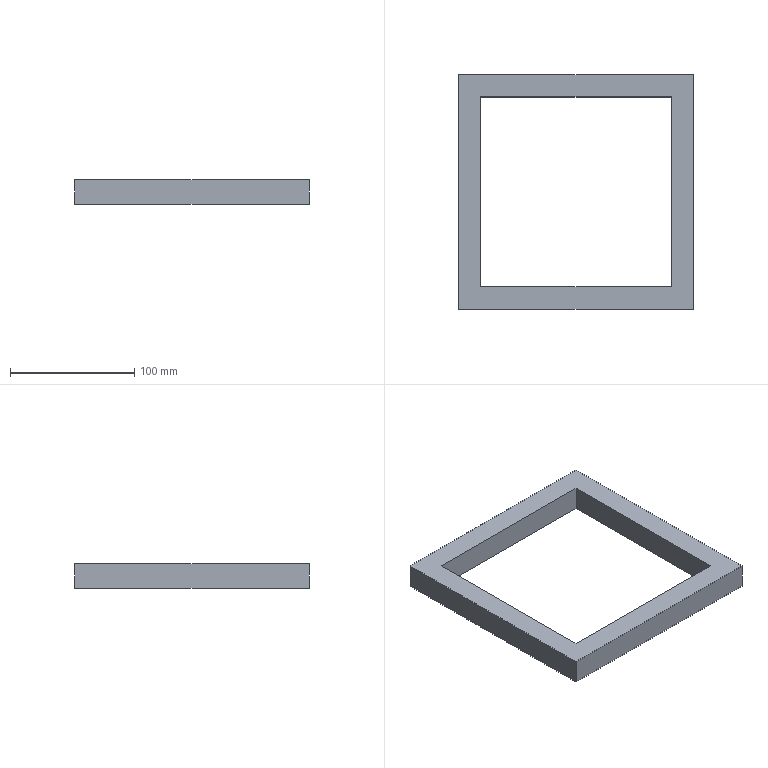Part | SolidWorks | features BaseBody 1 | 1 solid | 10 faces | box 189 x 189 x 20 mm | volume 246240 mm3 | plane 10
STEP:
#1=CARTESIAN_POINT('',(-76.5,-76.5,0.));
#2=VERTEX_POINT('',#1);
#3=CARTESIAN_POINT('',(76.5,-76.5,0.));
#4=VERTEX_POINT('',#3);
#5=CARTESIAN_POINT('',(76.5,-76.5,0.));
#6=DIRECTION('',(1.,0.,0.));
#7=VECTOR('',#6,1000.);
#8=LINE('',#5,#7);
#9=EDGE_CURVE('',#2,#4,#8,.T.);
#10=ORIENTED_EDGE('',*,*,#9,.F.);
#11=CARTESIAN_POINT('',(-76.5,-76.5,20.));
#12=VERTEX_POINT('',#11);
#13=CARTESIAN_POINT('',(-76.5,-76.5,20.));
#14=DIRECTION('',(0.,0.,-1.));
#15=VECTOR('',#14,1000.);
#16=LINE('',#13,#15);
#17=EDGE_CURVE('',#12,#2,#16,.T.);
#18=ORIENTED_EDGE('',*,*,#17,.F.);
#19=CARTESIAN_POINT('',(76.5,-76.5,20.));
#20=VERTEX_POINT('',#19);
#21=CARTESIAN_POINT('',(76.5,-76.5,20.));
#22=DIRECTION('',(1.,0.,0.));
#23=VECTOR('',#22,1000.);
#24=LINE('',#21,#23);
#25=EDGE_CURVE('',#12,#20,#24,.T.);
#26=ORIENTED_EDGE('',*,*,#25,.T.);
#27=CARTESIAN_POINT('',(76.5,-76.5,20.));
#28=DIRECTION('',(0.,0.,-1.));
#29=VECTOR('',#28,1000.);
#30=LINE('',#27,#29);
#31=EDGE_CURVE('',#20,#4,#30,.T.);
#32=ORIENTED_EDGE('',*,*,#31,.T.);
#33=EDGE_LOOP('',(#10,#18,#26,#32));
#34=FACE_OUTER_BOUND('',#33,.T.);
#35=CARTESIAN_POINT('',(76.5,-76.5,20.));
#36=DIRECTION('',(0.,1.,0.));
#37=DIRECTION('',(1.,0.,0.));
#38=AXIS2_PLACEMENT_3D('',#35,#36,#37);
#39=PLANE('',#38);
#40=ADVANCED_FACE('',(#34),#39,.T.);
#41=CARTESIAN_POINT('',(-76.5,76.5,0.));
#42=VERTEX_POINT('',#41);
#43=CARTESIAN_POINT('',(-76.5,76.5,0.));
#44=DIRECTION('',(0.,-1.,0.));
#45=VECTOR('',#44,1000.);
#46=LINE('',#43,#45);
#47=EDGE_CURVE('',#42,#2,#46,.T.);
#48=ORIENTED_EDGE('',*,*,#47,.F.);
#49=CARTESIAN_POINT('',(-76.5,76.5,20.));
#50=VERTEX_POINT('',#49);
#51=CARTESIAN_POINT('',(-76.5,76.5,20.));
#52=DIRECTION('',(0.,0.,-1.));
#53=VECTOR('',#52,1000.);
#54=LINE('',#51,#53);
#55=EDGE_CURVE('',#50,#42,#54,.T.);
#56=ORIENTED_EDGE('',*,*,#55,.F.);
#57=CARTESIAN_POINT('',(-76.5,76.5,20.));
#58=DIRECTION('',(0.,-1.,0.));
#59=VECTOR('',#58,1000.);
#60=LINE('',#57,#59);
#61=EDGE_CURVE('',#50,#12,#60,.T.);
#62=ORIENTED_EDGE('',*,*,#61,.T.);
#63=ORIENTED_EDGE('',*,*,#17,.T.);
#64=EDGE_LOOP('',(#48,#56,#62,#63));
#65=FACE_OUTER_BOUND('',#64,.T.);
#66=CARTESIAN_POINT('',(-76.5,76.5,20.));
#67=DIRECTION('',(1.,0.,0.));
#68=DIRECTION('',(0.,1.,0.));
#69=AXIS2_PLACEMENT_3D('',#66,#67,#68);
#70=PLANE('',#69);
#71=ADVANCED_FACE('',(#65),#70,.T.);
#72=CARTESIAN_POINT('',(76.5,76.5,0.));
#73=VERTEX_POINT('',#72);
#74=CARTESIAN_POINT('',(76.5,76.5,0.));
#75=DIRECTION('',(-1.,0.,0.));
#76=VECTOR('',#75,1000.);
#77=LINE('',#74,#76);
#78=EDGE_CURVE('',#73,#42,#77,.T.);
#79=ORIENTED_EDGE('',*,*,#78,.F.);
#80=CARTESIAN_POINT('',(76.5,76.5,20.));
#81=VERTEX_POINT('',#80);
#82=CARTESIAN_POINT('',(76.5,76.5,20.));
#83=DIRECTION('',(0.,0.,-1.));
#84=VECTOR('',#83,1000.);
#85=LINE('',#82,#84);
#86=EDGE_CURVE('',#81,#73,#85,.T.);
#87=ORIENTED_EDGE('',*,*,#86,.F.);
#88=CARTESIAN_POINT('',(76.5,76.5,20.));
#89=DIRECTION('',(-1.,0.,0.));
#90=VECTOR('',#89,1000.);
#91=LINE('',#88,#90);
#92=EDGE_CURVE('',#81,#50,#91,.T.);
#93=ORIENTED_EDGE('',*,*,#92,.T.);
#94=ORIENTED_EDGE('',*,*,#55,.T.);
#95=EDGE_LOOP('',(#79,#87,#93,#94));
#96=FACE_OUTER_BOUND('',#95,.T.);
#97=CARTESIAN_POINT('',(76.5,76.5,20.));
#98=DIRECTION('',(0.,-1.,0.));
#99=DIRECTION('',(0.,0.,-1.));
#100=AXIS2_PLACEMENT_3D('',#97,#98,#99);
#101=PLANE('',#100);
#102=ADVANCED_FACE('',(#96),#101,.T.);
#103=CARTESIAN_POINT('',(76.5,76.5,0.));
#104=DIRECTION('',(0.,1.,0.));
#105=VECTOR('',#104,1000.);
#106=LINE('',#103,#105);
#107=EDGE_CURVE('',#4,#73,#106,.T.);
#108=ORIENTED_EDGE('',*,*,#107,.F.);
#109=ORIENTED_EDGE('',*,*,#31,.F.);
#110=CARTESIAN_POINT('',(76.5,76.5,20.));
#111=DIRECTION('',(0.,1.,0.));
#112=VECTOR('',#111,1000.);
#113=LINE('',#110,#112);
#114=EDGE_CURVE('',#20,#81,#113,.T.);
#115=ORIENTED_EDGE('',*,*,#114,.T.);
#116=ORIENTED_EDGE('',*,*,#86,.T.);
#117=EDGE_LOOP('',(#108,#109,#115,#116));
#118=FACE_OUTER_BOUND('',#117,.T.);
#119=CARTESIAN_POINT('',(76.5,76.5,20.));
#120=DIRECTION('',(-1.,0.,0.));
#121=DIRECTION('',(0.,1.,0.));
#122=AXIS2_PLACEMENT_3D('',#119,#120,#121);
#123=PLANE('',#122);
#124=ADVANCED_FACE('',(#118),#123,.T.);
#125=CARTESIAN_POINT('',(94.5,94.5,0.));
#126=VERTEX_POINT('',#125);
#127=CARTESIAN_POINT('',(-94.5,94.5,0.));
#128=VERTEX_POINT('',#127);
#129=CARTESIAN_POINT('',(94.5,94.5,0.));
#130=DIRECTION('',(-1.,0.,0.));
#131=VECTOR('',#130,1000.);
#132=LINE('',#129,#131);
#133=EDGE_CURVE('',#126,#128,#132,.T.);
#134=ORIENTED_EDGE('',*,*,#133,.T.);
#135=CARTESIAN_POINT('',(-94.5,94.5,20.));
#136=VERTEX_POINT('',#135);
#137=CARTESIAN_POINT('',(-94.5,94.5,20.));
#138=DIRECTION('',(0.,0.,-1.));
#139=VECTOR('',#138,1000.);
#140=LINE('',#137,#139);
#141=EDGE_CURVE('',#136,#128,#140,.T.);
#142=ORIENTED_EDGE('',*,*,#141,.F.);
#143=CARTESIAN_POINT('',(94.5,94.5,20.));
#144=VERTEX_POINT('',#143);
#145=CARTESIAN_POINT('',(94.5,94.5,20.));
#146=DIRECTION('',(-1.,0.,0.));
#147=VECTOR('',#146,1000.);
#148=LINE('',#145,#147);
#149=EDGE_CURVE('',#144,#136,#148,.T.);
#150=ORIENTED_EDGE('',*,*,#149,.F.);
#151=CARTESIAN_POINT('',(94.5,94.5,20.));
#152=DIRECTION('',(0.,0.,-1.));
#153=VECTOR('',#152,1000.);
#154=LINE('',#151,#153);
#155=EDGE_CURVE('',#144,#126,#154,.T.);
#156=ORIENTED_EDGE('',*,*,#155,.T.);
#157=EDGE_LOOP('',(#134,#142,#150,#156));
#158=FACE_OUTER_BOUND('',#157,.T.);
#159=CARTESIAN_POINT('',(94.5,94.5,20.));
#160=DIRECTION('',(0.,-1.,0.));
#161=DIRECTION('',(0.,0.,-1.));
#162=AXIS2_PLACEMENT_3D('',#159,#160,#161);
#163=PLANE('',#162);
#164=ADVANCED_FACE('',(#158),#163,.F.);
#165=CARTESIAN_POINT('',(94.5,-94.5,0.));
#166=VERTEX_POINT('',#165);
#167=CARTESIAN_POINT('',(94.5,94.5,0.));
#168=DIRECTION('',(0.,1.,0.));
#169=VECTOR('',#168,1000.);
#170=LINE('',#167,#169);
#171=EDGE_CURVE('',#166,#126,#170,.T.);
#172=ORIENTED_EDGE('',*,*,#171,.T.);
#173=ORIENTED_EDGE('',*,*,#155,.F.);
#174=CARTESIAN_POINT('',(94.5,-94.5,20.));
#175=VERTEX_POINT('',#174);
#176=CARTESIAN_POINT('',(94.5,94.5,20.));
#177=DIRECTION('',(0.,1.,0.));
#178=VECTOR('',#177,1000.);
#179=LINE('',#176,#178);
#180=EDGE_CURVE('',#175,#144,#179,.T.);
#181=ORIENTED_EDGE('',*,*,#180,.F.);
#182=CARTESIAN_POINT('',(94.5,-94.5,20.));
#183=DIRECTION('',(0.,0.,-1.));
#184=VECTOR('',#183,1000.);
#185=LINE('',#182,#184);
#186=EDGE_CURVE('',#175,#166,#185,.T.);
#187=ORIENTED_EDGE('',*,*,#186,.T.);
#188=EDGE_LOOP('',(#172,#173,#181,#187));
#189=FACE_OUTER_BOUND('',#188,.T.);
#190=CARTESIAN_POINT('',(94.5,94.5,20.));
#191=DIRECTION('',(-1.,0.,0.));
#192=DIRECTION('',(0.,1.,0.));
#193=AXIS2_PLACEMENT_3D('',#190,#191,#192);
#194=PLANE('',#193);
#195=ADVANCED_FACE('',(#189),#194,.F.);
#196=CARTESIAN_POINT('',(-94.5,-94.5,0.));
#197=VERTEX_POINT('',#196);
#198=CARTESIAN_POINT('',(94.5,-94.5,0.));
#199=DIRECTION('',(1.,0.,0.));
#200=VECTOR('',#199,1000.);
#201=LINE('',#198,#200);
#202=EDGE_CURVE('',#197,#166,#201,.T.);
#203=ORIENTED_EDGE('',*,*,#202,.T.);
#204=ORIENTED_EDGE('',*,*,#186,.F.);
#205=CARTESIAN_POINT('',(-94.5,-94.5,20.));
#206=VERTEX_POINT('',#205);
#207=CARTESIAN_POINT('',(94.5,-94.5,20.));
#208=DIRECTION('',(1.,0.,0.));
#209=VECTOR('',#208,1000.);
#210=LINE('',#207,#209);
#211=EDGE_CURVE('',#206,#175,#210,.T.);
#212=ORIENTED_EDGE('',*,*,#211,.F.);
#213=CARTESIAN_POINT('',(-94.5,-94.5,20.));
#214=DIRECTION('',(0.,0.,-1.));
#215=VECTOR('',#214,1000.);
#216=LINE('',#213,#215);
#217=EDGE_CURVE('',#206,#197,#216,.T.);
#218=ORIENTED_EDGE('',*,*,#217,.T.);
#219=EDGE_LOOP('',(#203,#204,#212,#218));
#220=FACE_OUTER_BOUND('',#219,.T.);
#221=CARTESIAN_POINT('',(94.5,-94.5,20.));
#222=DIRECTION('',(0.,1.,0.));
#223=DIRECTION('',(1.,0.,0.));
#224=AXIS2_PLACEMENT_3D('',#221,#222,#223);
#225=PLANE('',#224);
#226=ADVANCED_FACE('',(#220),#225,.F.);
#227=CARTESIAN_POINT('',(-94.5,94.5,0.));
#228=DIRECTION('',(0.,-1.,0.));
#229=VECTOR('',#228,1000.);
#230=LINE('',#227,#229);
#231=EDGE_CURVE('',#128,#197,#230,.T.);
#232=ORIENTED_EDGE('',*,*,#231,.T.);
#233=ORIENTED_EDGE('',*,*,#217,.F.);
#234=CARTESIAN_POINT('',(-94.5,94.5,20.));
#235=DIRECTION('',(0.,-1.,0.));
#236=VECTOR('',#235,1000.);
#237=LINE('',#234,#236);
#238=EDGE_CURVE('',#136,#206,#237,.T.);
#239=ORIENTED_EDGE('',*,*,#238,.F.);
#240=ORIENTED_EDGE('',*,*,#141,.T.);
#241=EDGE_LOOP('',(#232,#233,#239,#240));
#242=FACE_OUTER_BOUND('',#241,.T.);
#243=CARTESIAN_POINT('',(-94.5,94.5,20.));
#244=DIRECTION('',(1.,0.,0.));
#245=DIRECTION('',(0.,1.,0.));
#246=AXIS2_PLACEMENT_3D('',#243,#244,#245);
#247=PLANE('',#246);
#248=ADVANCED_FACE('',(#242),#247,.F.);
#249=ORIENTED_EDGE('',*,*,#9,.T.);
#250=ORIENTED_EDGE('',*,*,#107,.T.);
#251=ORIENTED_EDGE('',*,*,#78,.T.);
#252=ORIENTED_EDGE('',*,*,#47,.T.);
#253=EDGE_LOOP('',(#249,#250,#251,#252));
#254=FACE_BOUND('',#253,.T.);
#255=ORIENTED_EDGE('',*,*,#231,.F.);
#256=ORIENTED_EDGE('',*,*,#133,.F.);
#257=ORIENTED_EDGE('',*,*,#171,.F.);
#258=ORIENTED_EDGE('',*,*,#202,.F.);
#259=EDGE_LOOP('',(#255,#256,#257,#258));
#260=FACE_OUTER_BOUND('',#259,.T.);
#261=CARTESIAN_POINT('',(0.,0.,0.));
#262=DIRECTION('',(0.,0.,-1.));
#263=DIRECTION('',(0.,-1.,0.));
#264=AXIS2_PLACEMENT_3D('',#261,#262,#263);
#265=PLANE('',#264);
#266=ADVANCED_FACE('',(#254,#260),#265,.T.);
#267=ORIENTED_EDGE('',*,*,#114,.F.);
#268=ORIENTED_EDGE('',*,*,#25,.F.);
#269=ORIENTED_EDGE('',*,*,#61,.F.);
#270=ORIENTED_EDGE('',*,*,#92,.F.);
#271=EDGE_LOOP('',(#267,#268,#269,#270));
#272=FACE_BOUND('',#271,.T.);
#273=ORIENTED_EDGE('',*,*,#238,.T.);
#274=ORIENTED_EDGE('',*,*,#211,.T.);
#275=ORIENTED_EDGE('',*,*,#180,.T.);
#276=ORIENTED_EDGE('',*,*,#149,.T.);
#277=EDGE_LOOP('',(#273,#274,#275,#276));
#278=FACE_OUTER_BOUND('',#277,.T.);
#279=CARTESIAN_POINT('',(0.,0.,20.));
#280=DIRECTION('',(0.,0.,-1.));
#281=DIRECTION('',(0.,-1.,0.));
#282=AXIS2_PLACEMENT_3D('',#279,#280,#281);
#283=PLANE('',#282);
#284=ADVANCED_FACE('',(#272,#278),#283,.F.);
#285=CLOSED_SHELL('',(#40,#71,#102,#124,#164,#195,#226,#248,#266,#284));
#286=MANIFOLD_SOLID_BREP('',#285);
#287=CARTESIAN_POINT('',(0.,0.,0.));
#288=DIRECTION('',(0.,0.,1.));
#289=DIRECTION('',(1.,0.,0.));
#290=AXIS2_PLACEMENT_3D('',#287,#288,#289);
#291=(LENGTH_UNIT()NAMED_UNIT(*)SI_UNIT(.MILLI.,.METRE.));
#292=UNCERTAINTY_MEASURE_WITH_UNIT(LENGTH_MEASURE(0.00001),#291,'','');
#293=(NAMED_UNIT(*)PLANE_ANGLE_UNIT()SI_UNIT($,.RADIAN.));
#294=(NAMED_UNIT(*)SI_UNIT($,.STERADIAN.)SOLID_ANGLE_UNIT());
#295=(GEOMETRIC_REPRESENTATION_CONTEXT(3)GLOBAL_UNCERTAINTY_ASSIGNED_CONTEXT((#292))GLOBAL_UNIT_ASSIGNED_CONTEXT((#291,#293,#294))REPRESENTATION_CONTEXT('',''));
#296=ADVANCED_BREP_SHAPE_REPRESENTATION('',(#286,#290),#295);